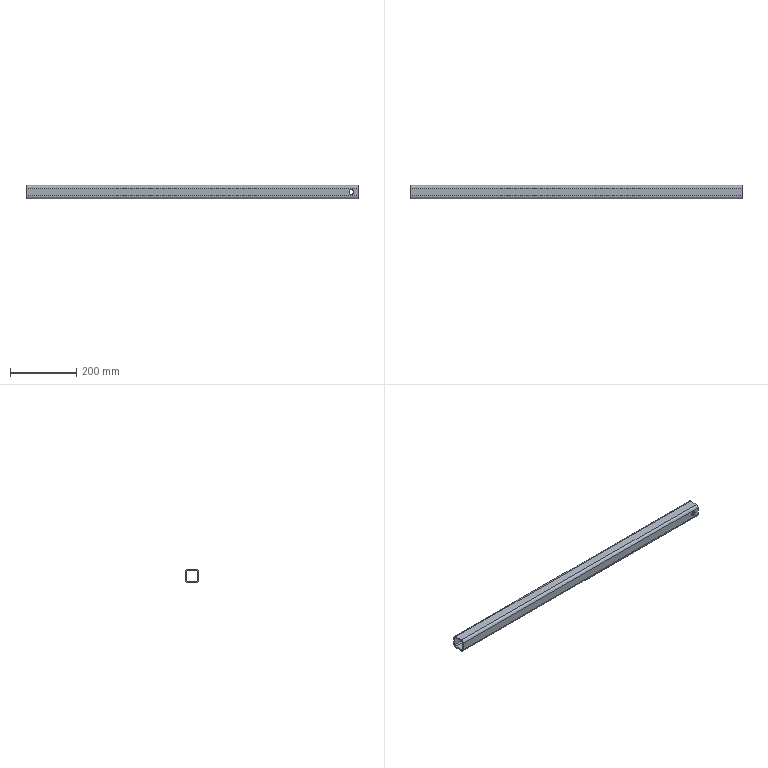Part | SolidWorks | features HoleWzd 1, ICE 1, WeldMemberFeat 1, WeldmentFeature 1 | 1 solid | 22 faces | box 1000 x 40 x 40 mm | volume 533565 mm3 | cylinder 12 | plane 10 | commonest cylinder face diameters 8 x4 14 x4 16 x4
STEP:
#1=CARTESIAN_POINT('',(-20.,16.,7.));
#2=VERTEX_POINT('',#1);
#3=CARTESIAN_POINT('',(-20.,16.,-7.));
#4=VERTEX_POINT('',#3);
#5=CARTESIAN_POINT('',(-20.,16.,0.));
#6=DIRECTION('',(0.,-1.,0.));
#7=DIRECTION('',(0.,0.,-1.));
#8=AXIS2_PLACEMENT_3D('',#5,#6,#7);
#9=CIRCLE('',#8,7.);
#10=EDGE_CURVE('',#2,#4,#9,.T.);
#11=ORIENTED_EDGE('',*,*,#10,.T.);
#12=CARTESIAN_POINT('',(-20.,20.,-7.));
#13=VERTEX_POINT('',#12);
#14=CARTESIAN_POINT('',(-20.,20.,-7.));
#15=DIRECTION('',(0.,1.,0.));
#16=VECTOR('',#15,1000.);
#17=LINE('',#14,#16);
#18=EDGE_CURVE('',#4,#13,#17,.T.);
#19=ORIENTED_EDGE('',*,*,#18,.T.);
#20=CARTESIAN_POINT('',(-20.,20.,7.));
#21=VERTEX_POINT('',#20);
#22=CARTESIAN_POINT('',(-20.,20.,0.));
#23=DIRECTION('',(0.,1.,0.));
#24=DIRECTION('',(0.,0.,1.));
#25=AXIS2_PLACEMENT_3D('',#22,#23,#24);
#26=CIRCLE('',#25,7.);
#27=EDGE_CURVE('',#13,#21,#26,.T.);
#28=ORIENTED_EDGE('',*,*,#27,.T.);
#29=CARTESIAN_POINT('',(-20.,20.,7.));
#30=DIRECTION('',(0.,1.,0.));
#31=VECTOR('',#30,1000.);
#32=LINE('',#29,#31);
#33=EDGE_CURVE('',#2,#21,#32,.T.);
#34=ORIENTED_EDGE('',*,*,#33,.F.);
#35=EDGE_LOOP('',(#11,#19,#28,#34));
#36=FACE_OUTER_BOUND('',#35,.T.);
#37=CARTESIAN_POINT('',(-20.,20.,0.));
#38=DIRECTION('',(0.,1.,0.));
#39=DIRECTION('',(0.,0.,1.));
#40=AXIS2_PLACEMENT_3D('',#37,#38,#39);
#41=CYLINDRICAL_SURFACE('',#40,7.);
#42=ADVANCED_FACE('',(#36),#41,.F.);
#43=CARTESIAN_POINT('',(-20.,-20.,-7.));
#44=VERTEX_POINT('',#43);
#45=CARTESIAN_POINT('',(-20.,-20.,7.));
#46=VERTEX_POINT('',#45);
#47=CARTESIAN_POINT('',(-20.,-20.,0.));
#48=DIRECTION('',(0.,1.,0.));
#49=DIRECTION('',(0.,0.,1.));
#50=AXIS2_PLACEMENT_3D('',#47,#48,#49);
#51=CIRCLE('',#50,7.);
#52=EDGE_CURVE('',#44,#46,#51,.T.);
#53=ORIENTED_EDGE('',*,*,#52,.F.);
#54=CARTESIAN_POINT('',(-20.,-16.,-7.));
#55=VERTEX_POINT('',#54);
#56=CARTESIAN_POINT('',(-20.,20.,-7.));
#57=DIRECTION('',(0.,1.,0.));
#58=VECTOR('',#57,1000.);
#59=LINE('',#56,#58);
#60=EDGE_CURVE('',#44,#55,#59,.T.);
#61=ORIENTED_EDGE('',*,*,#60,.T.);
#62=CARTESIAN_POINT('',(-20.,-16.,7.));
#63=VERTEX_POINT('',#62);
#64=CARTESIAN_POINT('',(-20.,-16.,0.));
#65=DIRECTION('',(0.,1.,0.));
#66=DIRECTION('',(0.,0.,1.));
#67=AXIS2_PLACEMENT_3D('',#64,#65,#66);
#68=CIRCLE('',#67,7.);
#69=EDGE_CURVE('',#55,#63,#68,.T.);
#70=ORIENTED_EDGE('',*,*,#69,.T.);
#71=CARTESIAN_POINT('',(-20.,20.,7.));
#72=DIRECTION('',(0.,1.,0.));
#73=VECTOR('',#72,1000.);
#74=LINE('',#71,#73);
#75=EDGE_CURVE('',#46,#63,#74,.T.);
#76=ORIENTED_EDGE('',*,*,#75,.F.);
#77=EDGE_LOOP('',(#53,#61,#70,#76));
#78=FACE_OUTER_BOUND('',#77,.T.);
#79=CARTESIAN_POINT('',(-20.,20.,0.));
#80=DIRECTION('',(0.,1.,0.));
#81=DIRECTION('',(0.,0.,1.));
#82=AXIS2_PLACEMENT_3D('',#79,#80,#81);
#83=CYLINDRICAL_SURFACE('',#82,7.);
#84=ADVANCED_FACE('',(#78),#83,.F.);
#85=CARTESIAN_POINT('',(0.,12.,20.));
#86=VERTEX_POINT('',#85);
#87=CARTESIAN_POINT('',(0.,20.,12.));
#88=VERTEX_POINT('',#87);
#89=CARTESIAN_POINT('',(0.,12.,12.));
#90=DIRECTION('',(-1.,0.,0.));
#91=DIRECTION('',(0.,0.,1.));
#92=AXIS2_PLACEMENT_3D('',#89,#90,#91);
#93=CIRCLE('',#92,8.);
#94=EDGE_CURVE('',#86,#88,#93,.T.);
#95=ORIENTED_EDGE('',*,*,#94,.T.);
#96=CARTESIAN_POINT('',(-1000.,20.,12.));
#97=VERTEX_POINT('',#96);
#98=CARTESIAN_POINT('',(-1000.,20.,12.));
#99=DIRECTION('',(1.,0.,0.));
#100=VECTOR('',#99,1000.);
#101=LINE('',#98,#100);
#102=EDGE_CURVE('',#97,#88,#101,.T.);
#103=ORIENTED_EDGE('',*,*,#102,.F.);
#104=CARTESIAN_POINT('',(-1000.,12.,20.));
#105=VERTEX_POINT('',#104);
#106=CARTESIAN_POINT('',(-1000.,12.,12.));
#107=DIRECTION('',(-1.,0.,0.));
#108=DIRECTION('',(0.,0.,1.));
#109=AXIS2_PLACEMENT_3D('',#106,#107,#108);
#110=CIRCLE('',#109,8.);
#111=EDGE_CURVE('',#105,#97,#110,.T.);
#112=ORIENTED_EDGE('',*,*,#111,.F.);
#113=CARTESIAN_POINT('',(-1000.,12.,20.));
#114=DIRECTION('',(1.,0.,0.));
#115=VECTOR('',#114,1000.);
#116=LINE('',#113,#115);
#117=EDGE_CURVE('',#105,#86,#116,.T.);
#118=ORIENTED_EDGE('',*,*,#117,.T.);
#119=EDGE_LOOP('',(#95,#103,#112,#118));
#120=FACE_OUTER_BOUND('',#119,.T.);
#121=CARTESIAN_POINT('',(-1000.,12.,12.));
#122=DIRECTION('',(1.,0.,0.));
#123=DIRECTION('',(0.,0.,-1.));
#124=AXIS2_PLACEMENT_3D('',#121,#122,#123);
#125=CYLINDRICAL_SURFACE('',#124,8.);
#126=ADVANCED_FACE('',(#120),#125,.T.);
#127=CARTESIAN_POINT('',(-20.,20.,0.));
#128=DIRECTION('',(0.,1.,0.));
#129=DIRECTION('',(0.,0.,1.));
#130=AXIS2_PLACEMENT_3D('',#127,#128,#129);
#131=CIRCLE('',#130,7.);
#132=EDGE_CURVE('',#21,#13,#131,.T.);
#133=ORIENTED_EDGE('',*,*,#132,.F.);
#134=ORIENTED_EDGE('',*,*,#27,.F.);
#135=EDGE_LOOP('',(#133,#134));
#136=FACE_BOUND('',#135,.T.);
#137=CARTESIAN_POINT('',(0.,20.,-12.));
#138=VERTEX_POINT('',#137);
#139=CARTESIAN_POINT('',(0.,20.,12.));
#140=DIRECTION('',(0.,0.,-1.));
#141=VECTOR('',#140,1000.);
#142=LINE('',#139,#141);
#143=EDGE_CURVE('',#88,#138,#142,.T.);
#144=ORIENTED_EDGE('',*,*,#143,.T.);
#145=CARTESIAN_POINT('',(-1000.,20.,-12.));
#146=VERTEX_POINT('',#145);
#147=CARTESIAN_POINT('',(-1000.,20.,-12.));
#148=DIRECTION('',(1.,0.,0.));
#149=VECTOR('',#148,1000.);
#150=LINE('',#147,#149);
#151=EDGE_CURVE('',#146,#138,#150,.T.);
#152=ORIENTED_EDGE('',*,*,#151,.F.);
#153=CARTESIAN_POINT('',(-1000.,20.,12.));
#154=DIRECTION('',(0.,0.,-1.));
#155=VECTOR('',#154,1000.);
#156=LINE('',#153,#155);
#157=EDGE_CURVE('',#97,#146,#156,.T.);
#158=ORIENTED_EDGE('',*,*,#157,.F.);
#159=ORIENTED_EDGE('',*,*,#102,.T.);
#160=EDGE_LOOP('',(#144,#152,#158,#159));
#161=FACE_OUTER_BOUND('',#160,.T.);
#162=CARTESIAN_POINT('',(-1000.,20.,12.));
#163=DIRECTION('',(0.,-1.,0.));
#164=DIRECTION('',(0.,0.,-1.));
#165=AXIS2_PLACEMENT_3D('',#162,#163,#164);
#166=PLANE('',#165);
#167=ADVANCED_FACE('',(#136,#161),#166,.F.);
#168=CARTESIAN_POINT('',(0.,12.,-20.));
#169=VERTEX_POINT('',#168);
#170=CARTESIAN_POINT('',(0.,12.,-12.));
#171=DIRECTION('',(-1.,0.,0.));
#172=DIRECTION('',(0.,0.,1.));
#173=AXIS2_PLACEMENT_3D('',#170,#171,#172);
#174=CIRCLE('',#173,8.);
#175=EDGE_CURVE('',#138,#169,#174,.T.);
#176=ORIENTED_EDGE('',*,*,#175,.T.);
#177=CARTESIAN_POINT('',(-1000.,12.,-20.));
#178=VERTEX_POINT('',#177);
#179=CARTESIAN_POINT('',(-1000.,12.,-20.));
#180=DIRECTION('',(1.,0.,0.));
#181=VECTOR('',#180,1000.);
#182=LINE('',#179,#181);
#183=EDGE_CURVE('',#178,#169,#182,.T.);
#184=ORIENTED_EDGE('',*,*,#183,.F.);
#185=CARTESIAN_POINT('',(-1000.,12.,-12.));
#186=DIRECTION('',(-1.,0.,0.));
#187=DIRECTION('',(0.,0.,1.));
#188=AXIS2_PLACEMENT_3D('',#185,#186,#187);
#189=CIRCLE('',#188,8.);
#190=EDGE_CURVE('',#146,#178,#189,.T.);
#191=ORIENTED_EDGE('',*,*,#190,.F.);
#192=ORIENTED_EDGE('',*,*,#151,.T.);
#193=EDGE_LOOP('',(#176,#184,#191,#192));
#194=FACE_OUTER_BOUND('',#193,.T.);
#195=CARTESIAN_POINT('',(-1000.,12.,-12.));
#196=DIRECTION('',(1.,0.,0.));
#197=DIRECTION('',(0.,0.,-1.));
#198=AXIS2_PLACEMENT_3D('',#195,#196,#197);
#199=CYLINDRICAL_SURFACE('',#198,8.);
#200=ADVANCED_FACE('',(#194),#199,.T.);
#201=CARTESIAN_POINT('',(0.,-12.,-20.));
#202=VERTEX_POINT('',#201);
#203=CARTESIAN_POINT('',(0.,-12.,-20.));
#204=DIRECTION('',(0.,-1.,0.));
#205=VECTOR('',#204,1000.);
#206=LINE('',#203,#205);
#207=EDGE_CURVE('',#169,#202,#206,.T.);
#208=ORIENTED_EDGE('',*,*,#207,.T.);
#209=CARTESIAN_POINT('',(-1000.,-12.,-20.));
#210=VERTEX_POINT('',#209);
#211=CARTESIAN_POINT('',(-1000.,-12.,-20.));
#212=DIRECTION('',(1.,0.,0.));
#213=VECTOR('',#212,1000.);
#214=LINE('',#211,#213);
#215=EDGE_CURVE('',#210,#202,#214,.T.);
#216=ORIENTED_EDGE('',*,*,#215,.F.);
#217=CARTESIAN_POINT('',(-1000.,-12.,-20.));
#218=DIRECTION('',(0.,-1.,0.));
#219=VECTOR('',#218,1000.);
#220=LINE('',#217,#219);
#221=EDGE_CURVE('',#178,#210,#220,.T.);
#222=ORIENTED_EDGE('',*,*,#221,.F.);
#223=ORIENTED_EDGE('',*,*,#183,.T.);
#224=EDGE_LOOP('',(#208,#216,#222,#223));
#225=FACE_OUTER_BOUND('',#224,.T.);
#226=CARTESIAN_POINT('',(-1000.,-12.,-20.));
#227=DIRECTION('',(0.,0.,1.));
#228=DIRECTION('',(1.,0.,0.));
#229=AXIS2_PLACEMENT_3D('',#226,#227,#228);
#230=PLANE('',#229);
#231=ADVANCED_FACE('',(#225),#230,.F.);
#232=CARTESIAN_POINT('',(0.,-20.,-12.));
#233=VERTEX_POINT('',#232);
#234=CARTESIAN_POINT('',(0.,-12.,-12.));
#235=DIRECTION('',(-1.,0.,0.));
#236=DIRECTION('',(0.,0.,1.));
#237=AXIS2_PLACEMENT_3D('',#234,#235,#236);
#238=CIRCLE('',#237,8.);
#239=EDGE_CURVE('',#202,#233,#238,.T.);
#240=ORIENTED_EDGE('',*,*,#239,.T.);
#241=CARTESIAN_POINT('',(-1000.,-20.,-12.));
#242=VERTEX_POINT('',#241);
#243=CARTESIAN_POINT('',(-1000.,-20.,-12.));
#244=DIRECTION('',(1.,0.,0.));
#245=VECTOR('',#244,1000.);
#246=LINE('',#243,#245);
#247=EDGE_CURVE('',#242,#233,#246,.T.);
#248=ORIENTED_EDGE('',*,*,#247,.F.);
#249=CARTESIAN_POINT('',(-1000.,-12.,-12.));
#250=DIRECTION('',(-1.,0.,0.));
#251=DIRECTION('',(0.,0.,1.));
#252=AXIS2_PLACEMENT_3D('',#249,#250,#251);
#253=CIRCLE('',#252,8.);
#254=EDGE_CURVE('',#210,#242,#253,.T.);
#255=ORIENTED_EDGE('',*,*,#254,.F.);
#256=ORIENTED_EDGE('',*,*,#215,.T.);
#257=EDGE_LOOP('',(#240,#248,#255,#256));
#258=FACE_OUTER_BOUND('',#257,.T.);
#259=CARTESIAN_POINT('',(-1000.,-12.,-12.));
#260=DIRECTION('',(1.,0.,0.));
#261=DIRECTION('',(0.,0.,-1.));
#262=AXIS2_PLACEMENT_3D('',#259,#260,#261);
#263=CYLINDRICAL_SURFACE('',#262,8.);
#264=ADVANCED_FACE('',(#258),#263,.T.);
#265=CARTESIAN_POINT('',(-20.,-20.,0.));
#266=DIRECTION('',(0.,1.,0.));
#267=DIRECTION('',(0.,0.,1.));
#268=AXIS2_PLACEMENT_3D('',#265,#266,#267);
#269=CIRCLE('',#268,7.);
#270=EDGE_CURVE('',#46,#44,#269,.T.);
#271=ORIENTED_EDGE('',*,*,#270,.T.);
#272=ORIENTED_EDGE('',*,*,#52,.T.);
#273=EDGE_LOOP('',(#271,#272));
#274=FACE_BOUND('',#273,.T.);
#275=CARTESIAN_POINT('',(0.,-20.,12.));
#276=VERTEX_POINT('',#275);
#277=CARTESIAN_POINT('',(0.,-20.,-12.));
#278=DIRECTION('',(0.,0.,1.));
#279=VECTOR('',#278,1000.);
#280=LINE('',#277,#279);
#281=EDGE_CURVE('',#233,#276,#280,.T.);
#282=ORIENTED_EDGE('',*,*,#281,.T.);
#283=CARTESIAN_POINT('',(-1000.,-20.,12.));
#284=VERTEX_POINT('',#283);
#285=CARTESIAN_POINT('',(-1000.,-20.,12.));
#286=DIRECTION('',(1.,0.,0.));
#287=VECTOR('',#286,1000.);
#288=LINE('',#285,#287);
#289=EDGE_CURVE('',#284,#276,#288,.T.);
#290=ORIENTED_EDGE('',*,*,#289,.F.);
#291=CARTESIAN_POINT('',(-1000.,-20.,-12.));
#292=DIRECTION('',(0.,0.,1.));
#293=VECTOR('',#292,1000.);
#294=LINE('',#291,#293);
#295=EDGE_CURVE('',#242,#284,#294,.T.);
#296=ORIENTED_EDGE('',*,*,#295,.F.);
#297=ORIENTED_EDGE('',*,*,#247,.T.);
#298=EDGE_LOOP('',(#282,#290,#296,#297));
#299=FACE_OUTER_BOUND('',#298,.T.);
#300=CARTESIAN_POINT('',(-1000.,-20.,-12.));
#301=DIRECTION('',(0.,1.,0.));
#302=DIRECTION('',(0.,0.,1.));
#303=AXIS2_PLACEMENT_3D('',#300,#301,#302);
#304=PLANE('',#303);
#305=ADVANCED_FACE('',(#274,#299),#304,.F.);
#306=CARTESIAN_POINT('',(0.,-12.,20.));
#307=VERTEX_POINT('',#306);
#308=CARTESIAN_POINT('',(0.,-12.,12.));
#309=DIRECTION('',(-1.,0.,0.));
#310=DIRECTION('',(0.,0.,1.));
#311=AXIS2_PLACEMENT_3D('',#308,#309,#310);
#312=CIRCLE('',#311,8.);
#313=EDGE_CURVE('',#276,#307,#312,.T.);
#314=ORIENTED_EDGE('',*,*,#313,.T.);
#315=CARTESIAN_POINT('',(-1000.,-12.,20.));
#316=VERTEX_POINT('',#315);
#317=CARTESIAN_POINT('',(-1000.,-12.,20.));
#318=DIRECTION('',(1.,0.,0.));
#319=VECTOR('',#318,1000.);
#320=LINE('',#317,#319);
#321=EDGE_CURVE('',#316,#307,#320,.T.);
#322=ORIENTED_EDGE('',*,*,#321,.F.);
#323=CARTESIAN_POINT('',(-1000.,-12.,12.));
#324=DIRECTION('',(-1.,0.,0.));
#325=DIRECTION('',(0.,0.,1.));
#326=AXIS2_PLACEMENT_3D('',#323,#324,#325);
#327=CIRCLE('',#326,8.);
#328=EDGE_CURVE('',#284,#316,#327,.T.);
#329=ORIENTED_EDGE('',*,*,#328,.F.);
#330=ORIENTED_EDGE('',*,*,#289,.T.);
#331=EDGE_LOOP('',(#314,#322,#329,#330));
#332=FACE_OUTER_BOUND('',#331,.T.);
#333=CARTESIAN_POINT('',(-1000.,-12.,12.));
#334=DIRECTION('',(1.,0.,0.));
#335=DIRECTION('',(0.,0.,-1.));
#336=AXIS2_PLACEMENT_3D('',#333,#334,#335);
#337=CYLINDRICAL_SURFACE('',#336,8.);
#338=ADVANCED_FACE('',(#332),#337,.T.);
#339=CARTESIAN_POINT('',(0.,16.,-12.));
#340=VERTEX_POINT('',#339);
#341=CARTESIAN_POINT('',(0.,12.,-16.));
#342=VERTEX_POINT('',#341);
#343=CARTESIAN_POINT('',(0.,12.,-12.));
#344=DIRECTION('',(-1.,0.,0.));
#345=DIRECTION('',(0.,0.,1.));
#346=AXIS2_PLACEMENT_3D('',#343,#344,#345);
#347=CIRCLE('',#346,4.);
#348=EDGE_CURVE('',#340,#342,#347,.T.);
#349=ORIENTED_EDGE('',*,*,#348,.F.);
#350=CARTESIAN_POINT('',(-1000.,16.,-12.));
#351=VERTEX_POINT('',#350);
#352=CARTESIAN_POINT('',(-1000.,16.,-12.));
#353=DIRECTION('',(1.,0.,0.));
#354=VECTOR('',#353,1000.);
#355=LINE('',#352,#354);
#356=EDGE_CURVE('',#351,#340,#355,.T.);
#357=ORIENTED_EDGE('',*,*,#356,.F.);
#358=CARTESIAN_POINT('',(-1000.,12.,-16.));
#359=VERTEX_POINT('',#358);
#360=CARTESIAN_POINT('',(-1000.,12.,-12.));
#361=DIRECTION('',(-1.,0.,0.));
#362=DIRECTION('',(0.,0.,1.));
#363=AXIS2_PLACEMENT_3D('',#360,#361,#362);
#364=CIRCLE('',#363,4.);
#365=EDGE_CURVE('',#351,#359,#364,.T.);
#366=ORIENTED_EDGE('',*,*,#365,.T.);
#367=CARTESIAN_POINT('',(-1000.,12.,-16.));
#368=DIRECTION('',(1.,0.,0.));
#369=VECTOR('',#368,1000.);
#370=LINE('',#367,#369);
#371=EDGE_CURVE('',#359,#342,#370,.T.);
#372=ORIENTED_EDGE('',*,*,#371,.T.);
#373=EDGE_LOOP('',(#349,#357,#366,#372));
#374=FACE_OUTER_BOUND('',#373,.T.);
#375=CARTESIAN_POINT('',(-1000.,12.,-12.));
#376=DIRECTION('',(1.,0.,0.));
#377=DIRECTION('',(0.,0.,-1.));
#378=AXIS2_PLACEMENT_3D('',#375,#376,#377);
#379=CYLINDRICAL_SURFACE('',#378,4.);
#380=ADVANCED_FACE('',(#374),#379,.F.);
#381=ORIENTED_EDGE('',*,*,#10,.F.);
#382=CARTESIAN_POINT('',(-20.,16.,0.));
#383=DIRECTION('',(0.,-1.,0.));
#384=DIRECTION('',(0.,0.,-1.));
#385=AXIS2_PLACEMENT_3D('',#382,#383,#384);
#386=CIRCLE('',#385,7.);
#387=EDGE_CURVE('',#4,#2,#386,.T.);
#388=ORIENTED_EDGE('',*,*,#387,.F.);
#389=EDGE_LOOP('',(#381,#388));
#390=FACE_BOUND('',#389,.T.);
#391=CARTESIAN_POINT('',(0.,16.,12.));
#392=VERTEX_POINT('',#391);
#393=CARTESIAN_POINT('',(0.,16.,12.));
#394=DIRECTION('',(0.,0.,-1.));
#395=VECTOR('',#394,1000.);
#396=LINE('',#393,#395);
#397=EDGE_CURVE('',#392,#340,#396,.T.);
#398=ORIENTED_EDGE('',*,*,#397,.F.);
#399=CARTESIAN_POINT('',(-1000.,16.,12.));
#400=VERTEX_POINT('',#399);
#401=CARTESIAN_POINT('',(-1000.,16.,12.));
#402=DIRECTION('',(1.,0.,0.));
#403=VECTOR('',#402,1000.);
#404=LINE('',#401,#403);
#405=EDGE_CURVE('',#400,#392,#404,.T.);
#406=ORIENTED_EDGE('',*,*,#405,.F.);
#407=CARTESIAN_POINT('',(-1000.,16.,12.));
#408=DIRECTION('',(0.,0.,-1.));
#409=VECTOR('',#408,1000.);
#410=LINE('',#407,#409);
#411=EDGE_CURVE('',#400,#351,#410,.T.);
#412=ORIENTED_EDGE('',*,*,#411,.T.);
#413=ORIENTED_EDGE('',*,*,#356,.T.);
#414=EDGE_LOOP('',(#398,#406,#412,#413));
#415=FACE_OUTER_BOUND('',#414,.T.);
#416=CARTESIAN_POINT('',(-1000.,16.,12.));
#417=DIRECTION('',(0.,-1.,0.));
#418=DIRECTION('',(0.,0.,-1.));
#419=AXIS2_PLACEMENT_3D('',#416,#417,#418);
#420=PLANE('',#419);
#421=ADVANCED_FACE('',(#390,#415),#420,.T.);
#422=CARTESIAN_POINT('',(0.,12.,16.));
#423=VERTEX_POINT('',#422);
#424=CARTESIAN_POINT('',(0.,12.,12.));
#425=DIRECTION('',(-1.,0.,0.));
#426=DIRECTION('',(0.,0.,1.));
#427=AXIS2_PLACEMENT_3D('',#424,#425,#426);
#428=CIRCLE('',#427,4.);
#429=EDGE_CURVE('',#423,#392,#428,.T.);
#430=ORIENTED_EDGE('',*,*,#429,.F.);
#431=CARTESIAN_POINT('',(-1000.,12.,16.));
#432=VERTEX_POINT('',#431);
#433=CARTESIAN_POINT('',(-1000.,12.,16.));
#434=DIRECTION('',(1.,0.,0.));
#435=VECTOR('',#434,1000.);
#436=LINE('',#433,#435);
#437=EDGE_CURVE('',#432,#423,#436,.T.);
#438=ORIENTED_EDGE('',*,*,#437,.F.);
#439=CARTESIAN_POINT('',(-1000.,12.,12.));
#440=DIRECTION('',(-1.,0.,0.));
#441=DIRECTION('',(0.,0.,1.));
#442=AXIS2_PLACEMENT_3D('',#439,#440,#441);
#443=CIRCLE('',#442,4.);
#444=EDGE_CURVE('',#432,#400,#443,.T.);
#445=ORIENTED_EDGE('',*,*,#444,.T.);
#446=ORIENTED_EDGE('',*,*,#405,.T.);
#447=EDGE_LOOP('',(#430,#438,#445,#446));
#448=FACE_OUTER_BOUND('',#447,.T.);
#449=CARTESIAN_POINT('',(-1000.,12.,12.));
#450=DIRECTION('',(1.,0.,0.));
#451=DIRECTION('',(0.,0.,-1.));
#452=AXIS2_PLACEMENT_3D('',#449,#450,#451);
#453=CYLINDRICAL_SURFACE('',#452,4.);
#454=ADVANCED_FACE('',(#448),#453,.F.);
#455=CARTESIAN_POINT('',(0.,-12.,16.));
#456=VERTEX_POINT('',#455);
#457=CARTESIAN_POINT('',(0.,12.,16.));
#458=DIRECTION('',(0.,1.,0.));
#459=VECTOR('',#458,1000.);
#460=LINE('',#457,#459);
#461=EDGE_CURVE('',#456,#423,#460,.T.);
#462=ORIENTED_EDGE('',*,*,#461,.F.);
#463=CARTESIAN_POINT('',(-1000.,-12.,16.));
#464=VERTEX_POINT('',#463);
#465=CARTESIAN_POINT('',(-1000.,-12.,16.));
#466=DIRECTION('',(1.,0.,0.));
#467=VECTOR('',#466,1000.);
#468=LINE('',#465,#467);
#469=EDGE_CURVE('',#464,#456,#468,.T.);
#470=ORIENTED_EDGE('',*,*,#469,.F.);
#471=CARTESIAN_POINT('',(-1000.,12.,16.));
#472=DIRECTION('',(0.,1.,0.));
#473=VECTOR('',#472,1000.);
#474=LINE('',#471,#473);
#475=EDGE_CURVE('',#464,#432,#474,.T.);
#476=ORIENTED_EDGE('',*,*,#475,.T.);
#477=ORIENTED_EDGE('',*,*,#437,.T.);
#478=EDGE_LOOP('',(#462,#470,#476,#477));
#479=FACE_OUTER_BOUND('',#478,.T.);
#480=CARTESIAN_POINT('',(-1000.,12.,16.));
#481=DIRECTION('',(0.,0.,-1.));
#482=DIRECTION('',(-1.,0.,0.));
#483=AXIS2_PLACEMENT_3D('',#480,#481,#482);
#484=PLANE('',#483);
#485=ADVANCED_FACE('',(#479),#484,.T.);
#486=CARTESIAN_POINT('',(0.,-16.,12.));
#487=VERTEX_POINT('',#486);
#488=CARTESIAN_POINT('',(0.,-12.,12.));
#489=DIRECTION('',(-1.,0.,0.));
#490=DIRECTION('',(0.,0.,1.));
#491=AXIS2_PLACEMENT_3D('',#488,#489,#490);
#492=CIRCLE('',#491,4.);
#493=EDGE_CURVE('',#487,#456,#492,.T.);
#494=ORIENTED_EDGE('',*,*,#493,.F.);
#495=CARTESIAN_POINT('',(-1000.,-16.,12.));
#496=VERTEX_POINT('',#495);
#497=CARTESIAN_POINT('',(-1000.,-16.,12.));
#498=DIRECTION('',(1.,0.,0.));
#499=VECTOR('',#498,1000.);
#500=LINE('',#497,#499);
#501=EDGE_CURVE('',#496,#487,#500,.T.);
#502=ORIENTED_EDGE('',*,*,#501,.F.);
#503=CARTESIAN_POINT('',(-1000.,-12.,12.));
#504=DIRECTION('',(-1.,0.,0.));
#505=DIRECTION('',(0.,0.,1.));
#506=AXIS2_PLACEMENT_3D('',#503,#504,#505);
#507=CIRCLE('',#506,4.);
#508=EDGE_CURVE('',#496,#464,#507,.T.);
#509=ORIENTED_EDGE('',*,*,#508,.T.);
#510=ORIENTED_EDGE('',*,*,#469,.T.);
#511=EDGE_LOOP('',(#494,#502,#509,#510));
#512=FACE_OUTER_BOUND('',#511,.T.);
#513=CARTESIAN_POINT('',(-1000.,-12.,12.));
#514=DIRECTION('',(1.,0.,0.));
#515=DIRECTION('',(0.,0.,-1.));
#516=AXIS2_PLACEMENT_3D('',#513,#514,#515);
#517=CYLINDRICAL_SURFACE('',#516,4.);
#518=ADVANCED_FACE('',(#512),#517,.F.);
#519=CARTESIAN_POINT('',(-20.,-16.,0.));
#520=DIRECTION('',(0.,1.,0.));
#521=DIRECTION('',(0.,0.,1.));
#522=AXIS2_PLACEMENT_3D('',#519,#520,#521);
#523=CIRCLE('',#522,7.);
#524=EDGE_CURVE('',#63,#55,#523,.T.);
#525=ORIENTED_EDGE('',*,*,#524,.F.);
#526=ORIENTED_EDGE('',*,*,#69,.F.);
#527=EDGE_LOOP('',(#525,#526));
#528=FACE_BOUND('',#527,.T.);
#529=CARTESIAN_POINT('',(0.,-16.,-12.));
#530=VERTEX_POINT('',#529);
#531=CARTESIAN_POINT('',(0.,-16.,-12.));
#532=DIRECTION('',(0.,0.,1.));
#533=VECTOR('',#532,1000.);
#534=LINE('',#531,#533);
#535=EDGE_CURVE('',#530,#487,#534,.T.);
#536=ORIENTED_EDGE('',*,*,#535,.F.);
#537=CARTESIAN_POINT('',(-1000.,-16.,-12.));
#538=VERTEX_POINT('',#537);
#539=CARTESIAN_POINT('',(-1000.,-16.,-12.));
#540=DIRECTION('',(1.,0.,0.));
#541=VECTOR('',#540,1000.);
#542=LINE('',#539,#541);
#543=EDGE_CURVE('',#538,#530,#542,.T.);
#544=ORIENTED_EDGE('',*,*,#543,.F.);
#545=CARTESIAN_POINT('',(-1000.,-16.,-12.));
#546=DIRECTION('',(0.,0.,1.));
#547=VECTOR('',#546,1000.);
#548=LINE('',#545,#547);
#549=EDGE_CURVE('',#538,#496,#548,.T.);
#550=ORIENTED_EDGE('',*,*,#549,.T.);
#551=ORIENTED_EDGE('',*,*,#501,.T.);
#552=EDGE_LOOP('',(#536,#544,#550,#551));
#553=FACE_OUTER_BOUND('',#552,.T.);
#554=CARTESIAN_POINT('',(-1000.,-16.,-12.));
#555=DIRECTION('',(0.,1.,0.));
#556=DIRECTION('',(0.,0.,1.));
#557=AXIS2_PLACEMENT_3D('',#554,#555,#556);
#558=PLANE('',#557);
#559=ADVANCED_FACE('',(#528,#553),#558,.T.);
#560=CARTESIAN_POINT('',(0.,-12.,-16.));
#561=VERTEX_POINT('',#560);
#562=CARTESIAN_POINT('',(0.,-12.,-12.));
#563=DIRECTION('',(-1.,0.,0.));
#564=DIRECTION('',(0.,0.,1.));
#565=AXIS2_PLACEMENT_3D('',#562,#563,#564);
#566=CIRCLE('',#565,4.);
#567=EDGE_CURVE('',#561,#530,#566,.T.);
#568=ORIENTED_EDGE('',*,*,#567,.F.);
#569=CARTESIAN_POINT('',(-1000.,-12.,-16.));
#570=VERTEX_POINT('',#569);
#571=CARTESIAN_POINT('',(-1000.,-12.,-16.));
#572=DIRECTION('',(1.,0.,0.));
#573=VECTOR('',#572,1000.);
#574=LINE('',#571,#573);
#575=EDGE_CURVE('',#570,#561,#574,.T.);
#576=ORIENTED_EDGE('',*,*,#575,.F.);
#577=CARTESIAN_POINT('',(-1000.,-12.,-12.));
#578=DIRECTION('',(-1.,0.,0.));
#579=DIRECTION('',(0.,0.,1.));
#580=AXIS2_PLACEMENT_3D('',#577,#578,#579);
#581=CIRCLE('',#580,4.);
#582=EDGE_CURVE('',#570,#538,#581,.T.);
#583=ORIENTED_EDGE('',*,*,#582,.T.);
#584=ORIENTED_EDGE('',*,*,#543,.T.);
#585=EDGE_LOOP('',(#568,#576,#583,#584));
#586=FACE_OUTER_BOUND('',#585,.T.);
#587=CARTESIAN_POINT('',(-1000.,-12.,-12.));
#588=DIRECTION('',(1.,0.,0.));
#589=DIRECTION('',(0.,0.,-1.));
#590=AXIS2_PLACEMENT_3D('',#587,#588,#589);
#591=CYLINDRICAL_SURFACE('',#590,4.);
#592=ADVANCED_FACE('',(#586),#591,.F.);
#593=CARTESIAN_POINT('',(0.,-12.,-16.));
#594=DIRECTION('',(0.,-1.,0.));
#595=VECTOR('',#594,1000.);
#596=LINE('',#593,#595);
#597=EDGE_CURVE('',#342,#561,#596,.T.);
#598=ORIENTED_EDGE('',*,*,#597,.F.);
#599=ORIENTED_EDGE('',*,*,#371,.F.);
#600=CARTESIAN_POINT('',(-1000.,-12.,-16.));
#601=DIRECTION('',(0.,-1.,0.));
#602=VECTOR('',#601,1000.);
#603=LINE('',#600,#602);
#604=EDGE_CURVE('',#359,#570,#603,.T.);
#605=ORIENTED_EDGE('',*,*,#604,.T.);
#606=ORIENTED_EDGE('',*,*,#575,.T.);
#607=EDGE_LOOP('',(#598,#599,#605,#606));
#608=FACE_OUTER_BOUND('',#607,.T.);
#609=CARTESIAN_POINT('',(-1000.,-12.,-16.));
#610=DIRECTION('',(0.,0.,1.));
#611=DIRECTION('',(1.,0.,0.));
#612=AXIS2_PLACEMENT_3D('',#609,#610,#611);
#613=PLANE('',#612);
#614=ADVANCED_FACE('',(#608),#613,.T.);
#615=CARTESIAN_POINT('',(0.,12.,20.));
#616=DIRECTION('',(0.,1.,0.));
#617=VECTOR('',#616,1000.);
#618=LINE('',#615,#617);
#619=EDGE_CURVE('',#307,#86,#618,.T.);
#620=ORIENTED_EDGE('',*,*,#619,.T.);
#621=ORIENTED_EDGE('',*,*,#117,.F.);
#622=CARTESIAN_POINT('',(-1000.,12.,20.));
#623=DIRECTION('',(0.,1.,0.));
#624=VECTOR('',#623,1000.);
#625=LINE('',#622,#624);
#626=EDGE_CURVE('',#316,#105,#625,.T.);
#627=ORIENTED_EDGE('',*,*,#626,.F.);
#628=ORIENTED_EDGE('',*,*,#321,.T.);
#629=EDGE_LOOP('',(#620,#621,#627,#628));
#630=FACE_OUTER_BOUND('',#629,.T.);
#631=CARTESIAN_POINT('',(-1000.,12.,20.));
#632=DIRECTION('',(0.,0.,-1.));
#633=DIRECTION('',(-1.,0.,0.));
#634=AXIS2_PLACEMENT_3D('',#631,#632,#633);
#635=PLANE('',#634);
#636=ADVANCED_FACE('',(#630),#635,.F.);
#637=ORIENTED_EDGE('',*,*,#365,.F.);
#638=ORIENTED_EDGE('',*,*,#411,.F.);
#639=ORIENTED_EDGE('',*,*,#444,.F.);
#640=ORIENTED_EDGE('',*,*,#475,.F.);
#641=ORIENTED_EDGE('',*,*,#508,.F.);
#642=ORIENTED_EDGE('',*,*,#549,.F.);
#643=ORIENTED_EDGE('',*,*,#582,.F.);
#644=ORIENTED_EDGE('',*,*,#604,.F.);
#645=EDGE_LOOP('',(#637,#638,#639,#640,#641,#642,#643,#644));
#646=FACE_BOUND('',#645,.T.);
#647=ORIENTED_EDGE('',*,*,#111,.T.);
#648=ORIENTED_EDGE('',*,*,#157,.T.);
#649=ORIENTED_EDGE('',*,*,#190,.T.);
#650=ORIENTED_EDGE('',*,*,#221,.T.);
#651=ORIENTED_EDGE('',*,*,#254,.T.);
#652=ORIENTED_EDGE('',*,*,#295,.T.);
#653=ORIENTED_EDGE('',*,*,#328,.T.);
#654=ORIENTED_EDGE('',*,*,#626,.T.);
#655=EDGE_LOOP('',(#647,#648,#649,#650,#651,#652,#653,#654));
#656=FACE_OUTER_BOUND('',#655,.T.);
#657=CARTESIAN_POINT('',(-1000.,12.,12.));
#658=DIRECTION('',(-1.,0.,0.));
#659=DIRECTION('',(0.,0.,1.));
#660=AXIS2_PLACEMENT_3D('',#657,#658,#659);
#661=PLANE('',#660);
#662=ADVANCED_FACE('',(#646,#656),#661,.T.);
#663=ORIENTED_EDGE('',*,*,#348,.T.);
#664=ORIENTED_EDGE('',*,*,#597,.T.);
#665=ORIENTED_EDGE('',*,*,#567,.T.);
#666=ORIENTED_EDGE('',*,*,#535,.T.);
#667=ORIENTED_EDGE('',*,*,#493,.T.);
#668=ORIENTED_EDGE('',*,*,#461,.T.);
#669=ORIENTED_EDGE('',*,*,#429,.T.);
#670=ORIENTED_EDGE('',*,*,#397,.T.);
#671=EDGE_LOOP('',(#663,#664,#665,#666,#667,#668,#669,#670));
#672=FACE_BOUND('',#671,.T.);
#673=ORIENTED_EDGE('',*,*,#94,.F.);
#674=ORIENTED_EDGE('',*,*,#619,.F.);
#675=ORIENTED_EDGE('',*,*,#313,.F.);
#676=ORIENTED_EDGE('',*,*,#281,.F.);
#677=ORIENTED_EDGE('',*,*,#239,.F.);
#678=ORIENTED_EDGE('',*,*,#207,.F.);
#679=ORIENTED_EDGE('',*,*,#175,.F.);
#680=ORIENTED_EDGE('',*,*,#143,.F.);
#681=EDGE_LOOP('',(#673,#674,#675,#676,#677,#678,#679,#680));
#682=FACE_OUTER_BOUND('',#681,.T.);
#683=CARTESIAN_POINT('',(0.,12.,12.));
#684=DIRECTION('',(-1.,0.,0.));
#685=DIRECTION('',(0.,0.,1.));
#686=AXIS2_PLACEMENT_3D('',#683,#684,#685);
#687=PLANE('',#686);
#688=ADVANCED_FACE('',(#672,#682),#687,.F.);
#689=ORIENTED_EDGE('',*,*,#60,.F.);
#690=ORIENTED_EDGE('',*,*,#270,.F.);
#691=ORIENTED_EDGE('',*,*,#75,.T.);
#692=ORIENTED_EDGE('',*,*,#524,.T.);
#693=EDGE_LOOP('',(#689,#690,#691,#692));
#694=FACE_OUTER_BOUND('',#693,.T.);
#695=CARTESIAN_POINT('',(-20.,20.,0.));
#696=DIRECTION('',(0.,1.,0.));
#697=DIRECTION('',(0.,0.,1.));
#698=AXIS2_PLACEMENT_3D('',#695,#696,#697);
#699=CYLINDRICAL_SURFACE('',#698,7.);
#700=ADVANCED_FACE('',(#694),#699,.F.);
#701=ORIENTED_EDGE('',*,*,#18,.F.);
#702=ORIENTED_EDGE('',*,*,#387,.T.);
#703=ORIENTED_EDGE('',*,*,#33,.T.);
#704=ORIENTED_EDGE('',*,*,#132,.T.);
#705=EDGE_LOOP('',(#701,#702,#703,#704));
#706=FACE_OUTER_BOUND('',#705,.T.);
#707=CARTESIAN_POINT('',(-20.,20.,0.));
#708=DIRECTION('',(0.,1.,0.));
#709=DIRECTION('',(0.,0.,1.));
#710=AXIS2_PLACEMENT_3D('',#707,#708,#709);
#711=CYLINDRICAL_SURFACE('',#710,7.);
#712=ADVANCED_FACE('',(#706),#711,.F.);
#713=CLOSED_SHELL('',(#42,#84,#126,#167,#200,#231,#264,#305,#338,#380,#421,#454,#485,#518,#559,#592,#614,#636,#662,#688,#700,#712));
#714=MANIFOLD_SOLID_BREP('',#713);
#715=CARTESIAN_POINT('',(0.,0.,0.));
#716=DIRECTION('',(0.,0.,1.));
#717=DIRECTION('',(1.,0.,0.));
#718=AXIS2_PLACEMENT_3D('',#715,#716,#717);
#719=(LENGTH_UNIT()NAMED_UNIT(*)SI_UNIT(.MILLI.,.METRE.));
#720=UNCERTAINTY_MEASURE_WITH_UNIT(LENGTH_MEASURE(0.00001),#719,'','');
#721=(NAMED_UNIT(*)PLANE_ANGLE_UNIT()SI_UNIT($,.RADIAN.));
#722=(NAMED_UNIT(*)SI_UNIT($,.STERADIAN.)SOLID_ANGLE_UNIT());
#723=(GEOMETRIC_REPRESENTATION_CONTEXT(3)GLOBAL_UNCERTAINTY_ASSIGNED_CONTEXT((#720))GLOBAL_UNIT_ASSIGNED_CONTEXT((#719,#721,#722))REPRESENTATION_CONTEXT('',''));
#724=ADVANCED_BREP_SHAPE_REPRESENTATION('',(#714,#718),#723);